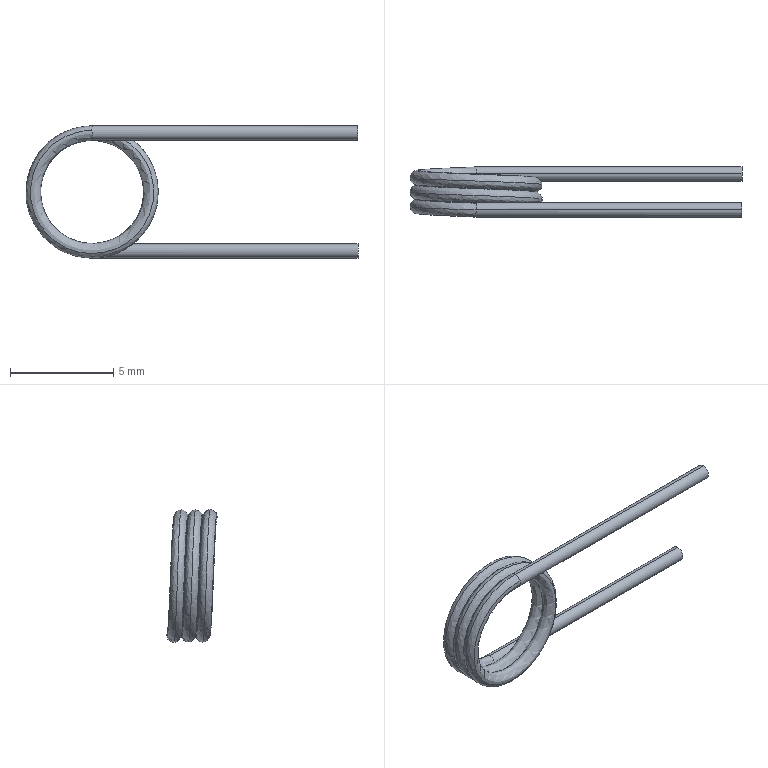Part | SolidWorks | features CompositeCurve 1, Helix 1, Sweep 1 | 1 solid | 9 faces | box 16.05 x 2.45 x 6.4 mm | volume 26.63 mm3 | cylinder 4 | spline 3 | plane 2 | commonest cylinder face diameters 0.7 x4
STEP:
#1=CARTESIAN_POINT('',(12.85,1.75,-3.2));
#2=VERTEX_POINT('',#1);
#3=CARTESIAN_POINT('',(12.85,1.75,-2.5));
#4=VERTEX_POINT('',#3);
#5=CARTESIAN_POINT('',(12.85,1.75,-2.85));
#6=DIRECTION('',(1.,0.,0.));
#7=DIRECTION('',(0.,0.00009155,-1.));
#8=AXIS2_PLACEMENT_3D('',#5,#6,#7);
#9=CIRCLE('',#8,0.35);
#10=EDGE_CURVE('',#2,#4,#9,.T.);
#11=ORIENTED_EDGE('',*,*,#10,.F.);
#12=CARTESIAN_POINT('',(-0.000000536,1.75,-3.2));
#13=VERTEX_POINT('',#12);
#14=CARTESIAN_POINT('',(12.85,1.75,-3.2));
#15=DIRECTION('',(-1.,0.,0.));
#16=VECTOR('',#15,1000.);
#17=LINE('',#14,#16);
#18=EDGE_CURVE('',#2,#13,#17,.T.);
#19=ORIENTED_EDGE('',*,*,#18,.T.);
#20=CARTESIAN_POINT('',(-0.006305,2.074,-2.979));
#21=VERTEX_POINT('',#20);
#22=CARTESIAN_POINT('',(0.,1.75,-2.85));
#23=DIRECTION('',(1.,0.,0.));
#24=DIRECTION('',(0.,0.00009155,-1.));
#25=AXIS2_PLACEMENT_3D('',#22,#23,#24);
#26=CIRCLE('',#25,0.35);
#27=EDGE_CURVE('',#13,#21,#26,.T.);
#28=ORIENTED_EDGE('',*,*,#27,.T.);
#29=CARTESIAN_POINT('',(0.,1.75,-2.5));
#30=VERTEX_POINT('',#29);
#31=CARTESIAN_POINT('',(0.,1.75,-2.85));
#32=DIRECTION('',(1.,0.,0.));
#33=DIRECTION('',(0.,0.00009155,-1.));
#34=AXIS2_PLACEMENT_3D('',#31,#32,#33);
#35=CIRCLE('',#34,0.35);
#36=EDGE_CURVE('',#21,#30,#35,.T.);
#37=ORIENTED_EDGE('',*,*,#36,.T.);
#38=CARTESIAN_POINT('',(12.85,1.75,-2.5));
#39=DIRECTION('',(-1.,0.,0.));
#40=VECTOR('',#39,1000.);
#41=LINE('',#38,#40);
#42=EDGE_CURVE('',#4,#30,#41,.T.);
#43=ORIENTED_EDGE('',*,*,#42,.F.);
#44=EDGE_LOOP('',(#11,#19,#28,#37,#43));
#45=FACE_OUTER_BOUND('',#44,.T.);
#46=CARTESIAN_POINT('',(12.85,1.75,-2.85));
#47=DIRECTION('',(-1.,0.,0.));
#48=DIRECTION('',(0.,0.,1.));
#49=AXIS2_PLACEMENT_3D('',#46,#47,#48);
#50=CYLINDRICAL_SURFACE('',#49,0.35);
#51=ADVANCED_FACE('',(#45),#50,.T.);
#52=CARTESIAN_POINT('',(0.006305,0.3239,2.979));
#53=VERTEX_POINT('',#52);
#54=CARTESIAN_POINT('',(0.,0.,3.2));
#55=VERTEX_POINT('',#54);
#56=CARTESIAN_POINT('',(0.006305,0.3239,2.979));
#57=CARTESIAN_POINT('',(0.01048,0.2681,3.104));
#58=CARTESIAN_POINT('',(0.005425,0.1388,3.2));
#59=CARTESIAN_POINT('',(0.,0.,3.2));
#60=B_SPLINE_CURVE_WITH_KNOTS('',3,(#56,#57,#58,#59),.UNSPECIFIED.,.F.,.F.,(4,4),(0.00002721,0.1895),.UNSPECIFIED.);
#61=EDGE_CURVE('',#53,#55,#60,.T.);
#62=ORIENTED_EDGE('',*,*,#61,.T.);
#63=CARTESIAN_POINT('',(12.85,0.,3.2));
#64=VERTEX_POINT('',#63);
#65=CARTESIAN_POINT('',(0.,0.,3.2));
#66=DIRECTION('',(1.,0.,0.));
#67=VECTOR('',#66,1000.);
#68=LINE('',#65,#67);
#69=EDGE_CURVE('',#55,#64,#68,.T.);
#70=ORIENTED_EDGE('',*,*,#69,.T.);
#71=CARTESIAN_POINT('',(12.85,0.,2.5));
#72=VERTEX_POINT('',#71);
#73=CARTESIAN_POINT('',(12.85,0.,2.85));
#74=DIRECTION('',(-1.,0.,0.));
#75=DIRECTION('',(0.,0.,1.));
#76=AXIS2_PLACEMENT_3D('',#73,#74,#75);
#77=CIRCLE('',#76,0.35);
#78=EDGE_CURVE('',#64,#72,#77,.T.);
#79=ORIENTED_EDGE('',*,*,#78,.T.);
#80=CARTESIAN_POINT('',(0.,0.,2.5));
#81=VERTEX_POINT('',#80);
#82=CARTESIAN_POINT('',(0.,0.,2.5));
#83=DIRECTION('',(1.,0.,0.));
#84=VECTOR('',#83,1000.);
#85=LINE('',#82,#84);
#86=EDGE_CURVE('',#81,#72,#85,.T.);
#87=ORIENTED_EDGE('',*,*,#86,.F.);
#88=CARTESIAN_POINT('',(0.,0.,2.85));
#89=DIRECTION('',(-1.,0.,0.));
#90=DIRECTION('',(0.,0.,1.));
#91=AXIS2_PLACEMENT_3D('',#88,#89,#90);
#92=CIRCLE('',#91,0.35);
#93=EDGE_CURVE('',#53,#81,#92,.T.);
#94=ORIENTED_EDGE('',*,*,#93,.F.);
#95=EDGE_LOOP('',(#62,#70,#79,#87,#94));
#96=FACE_OUTER_BOUND('',#95,.T.);
#97=CARTESIAN_POINT('',(0.,0.,2.85));
#98=DIRECTION('',(1.,0.,0.));
#99=DIRECTION('',(0.,0.,-1.));
#100=AXIS2_PLACEMENT_3D('',#97,#98,#99);
#101=CYLINDRICAL_SURFACE('',#100,0.35);
#102=ADVANCED_FACE('',(#96),#101,.T.);
#103=ORIENTED_EDGE('',*,*,#18,.F.);
#104=CARTESIAN_POINT('',(12.85,1.75,-2.85));
#105=DIRECTION('',(1.,0.,0.));
#106=DIRECTION('',(0.,0.00009155,-1.));
#107=AXIS2_PLACEMENT_3D('',#104,#105,#106);
#108=CIRCLE('',#107,0.35);
#109=EDGE_CURVE('',#4,#2,#108,.T.);
#110=ORIENTED_EDGE('',*,*,#109,.F.);
#111=ORIENTED_EDGE('',*,*,#42,.T.);
#112=CARTESIAN_POINT('',(0.006304,1.426,-2.979));
#113=VERTEX_POINT('',#112);
#114=CARTESIAN_POINT('',(0.,1.75,-2.85));
#115=DIRECTION('',(1.,0.,0.));
#116=DIRECTION('',(0.,0.00009155,-1.));
#117=AXIS2_PLACEMENT_3D('',#114,#115,#116);
#118=CIRCLE('',#117,0.35);
#119=EDGE_CURVE('',#30,#113,#118,.T.);
#120=ORIENTED_EDGE('',*,*,#119,.T.);
#121=CARTESIAN_POINT('',(0.,1.75,-2.85));
#122=DIRECTION('',(1.,0.,0.));
#123=DIRECTION('',(0.,0.00009155,-1.));
#124=AXIS2_PLACEMENT_3D('',#121,#122,#123);
#125=CIRCLE('',#124,0.35);
#126=EDGE_CURVE('',#113,#13,#125,.T.);
#127=ORIENTED_EDGE('',*,*,#126,.T.);
#128=EDGE_LOOP('',(#103,#110,#111,#120,#127));
#129=FACE_OUTER_BOUND('',#128,.T.);
#130=CARTESIAN_POINT('',(12.85,1.75,-2.85));
#131=DIRECTION('',(-1.,0.,0.));
#132=DIRECTION('',(0.,0.,1.));
#133=AXIS2_PLACEMENT_3D('',#130,#131,#132);
#134=CYLINDRICAL_SURFACE('',#133,0.35);
#135=ADVANCED_FACE('',(#129),#134,.T.);
#136=ORIENTED_EDGE('',*,*,#36,.F.);
#137=CARTESIAN_POINT('',(0.006305,0.3239,2.979));
#138=CARTESIAN_POINT('',(-0.7712,0.3519,2.981));
#139=CARTESIAN_POINT('',(-1.545,0.381,2.663));
#140=CARTESIAN_POINT('',(-2.649,0.4392,1.566));
#141=CARTESIAN_POINT('',(-2.975,0.4683,0.7939));
#142=CARTESIAN_POINT('',(-2.98,0.5195,-0.5733));
#143=CARTESIAN_POINT('',(-2.806,0.5413,-1.156));
#144=CARTESIAN_POINT('',(-2.162,0.585,-2.13));
#145=CARTESIAN_POINT('',(-1.69,0.6069,-2.521));
#146=CARTESIAN_POINT('',(-0.4324,0.658,-3.048));
#147=CARTESIAN_POINT('',(0.405,0.6871,-3.052));
#148=CARTESIAN_POINT('',(1.67,0.7383,-2.534));
#149=CARTESIAN_POINT('',(2.142,0.7601,-2.15));
#150=CARTESIAN_POINT('',(2.795,0.8037,-1.182));
#151=CARTESIAN_POINT('',(2.976,0.8257,-0.5972));
#152=CARTESIAN_POINT('',(2.981,0.8768,0.7668));
#153=CARTESIAN_POINT('',(2.665,0.9058,1.542));
#154=CARTESIAN_POINT('',(1.702,0.957,2.513));
#155=CARTESIAN_POINT('',(1.167,0.9788,2.801));
#156=CARTESIAN_POINT('',(0.02248,1.022,3.035));
#157=CARTESIAN_POINT('',(-0.587,1.044,2.978));
#158=CARTESIAN_POINT('',(-1.849,1.096,2.461));
#159=CARTESIAN_POINT('',(-2.445,1.125,1.872));
#160=CARTESIAN_POINT('',(-2.973,1.176,0.6109));
#161=CARTESIAN_POINT('',(-3.035,1.198,0.005944));
#162=CARTESIAN_POINT('',(-2.812,1.241,-1.14));
#163=CARTESIAN_POINT('',(-2.526,1.263,-1.682));
#164=CARTESIAN_POINT('',(-1.566,1.314,-2.65));
#165=CARTESIAN_POINT('',(-0.7938,1.343,-2.975));
#166=CARTESIAN_POINT('',(0.5733,1.395,-2.98));
#167=CARTESIAN_POINT('',(1.156,1.416,-2.806));
#168=CARTESIAN_POINT('',(2.13,1.46,-2.162));
#169=CARTESIAN_POINT('',(2.521,1.482,-1.69));
#170=CARTESIAN_POINT('',(3.048,1.533,-0.4324));
#171=CARTESIAN_POINT('',(3.052,1.562,0.405));
#172=CARTESIAN_POINT('',(2.534,1.613,1.67));
#173=CARTESIAN_POINT('',(2.15,1.635,2.142));
#174=CARTESIAN_POINT('',(1.182,1.679,2.795));
#175=CARTESIAN_POINT('',(0.5972,1.701,2.976));
#176=CARTESIAN_POINT('',(-0.7668,1.752,2.981));
#177=CARTESIAN_POINT('',(-1.542,1.781,2.665));
#178=CARTESIAN_POINT('',(-2.513,1.832,1.702));
#179=CARTESIAN_POINT('',(-2.801,1.854,1.167));
#180=CARTESIAN_POINT('',(-3.034,1.897,0.0225));
#181=CARTESIAN_POINT('',(-2.978,1.919,-0.587));
#182=CARTESIAN_POINT('',(-2.46,1.971,-1.85));
#183=CARTESIAN_POINT('',(-1.872,2.,-2.445));
#184=CARTESIAN_POINT('',(-0.7917,2.043,-2.897));
#185=CARTESIAN_POINT('',(-0.4042,2.058,-2.976));
#186=CARTESIAN_POINT('',(-0.006305,2.074,-2.979));
#187=B_SPLINE_CURVE_WITH_KNOTS('',3,(#137,#138,#139,#140,#141,#142,#143,#144,#145,#146,#147,#148,#149,#150,#151,#152,#153,#154,#155,#156,#157,#158,#159,#160,#161,#162,#163,#164,#165,#166,#167,#168,#169,#170,#171,#172,#173,#174,#175,#176,#177,#178,#179,#180,#181,#182,#183,#184,#185,#186),.UNSPECIFIED.,.F.,.F.,(4,2,2,2,2,2,2,2,2,2,2,2,2,2,2,2,2,2,2,2,2,2,2,2,4),(0.,0.04998,0.09999,0.1375,0.175,0.225,0.2625,0.3,0.35,0.3875,0.425,0.475,0.5125,0.55,0.6,0.6375,0.675,0.725,0.7625,0.8,0.85,0.8875,0.925,0.975,1.),.UNSPECIFIED.);
#188=EDGE_CURVE('',#53,#21,#187,.T.);
#189=ORIENTED_EDGE('',*,*,#188,.F.);
#190=ORIENTED_EDGE('',*,*,#93,.T.);
#191=CARTESIAN_POINT('',(-0.006304,-0.3239,2.979));
#192=VERTEX_POINT('',#191);
#193=CARTESIAN_POINT('',(0.,0.,2.85));
#194=DIRECTION('',(-1.,0.,0.));
#195=DIRECTION('',(0.,0.,1.));
#196=AXIS2_PLACEMENT_3D('',#193,#194,#195);
#197=CIRCLE('',#196,0.35);
#198=EDGE_CURVE('',#81,#192,#197,.T.);
#199=ORIENTED_EDGE('',*,*,#198,.T.);
#200=CARTESIAN_POINT('',(0.006304,1.426,-2.979));
#201=CARTESIAN_POINT('',(-0.379,1.413,-2.98));
#202=CARTESIAN_POINT('',(-0.7673,1.398,-2.904));
#203=CARTESIAN_POINT('',(-1.851,1.354,-2.461));
#204=CARTESIAN_POINT('',(-2.445,1.325,-1.871));
#205=CARTESIAN_POINT('',(-2.973,1.274,-0.6122));
#206=CARTESIAN_POINT('',(-3.035,1.252,-0.003211));
#207=CARTESIAN_POINT('',(-2.811,1.209,1.143));
#208=CARTESIAN_POINT('',(-2.527,1.187,1.681));
#209=CARTESIAN_POINT('',(-1.565,1.136,2.652));
#210=CARTESIAN_POINT('',(-0.792,1.107,2.975));
#211=CARTESIAN_POINT('',(0.572,1.056,2.981));
#212=CARTESIAN_POINT('',(1.158,1.034,2.805));
#213=CARTESIAN_POINT('',(2.132,0.99,2.16));
#214=CARTESIAN_POINT('',(2.52,0.9682,1.692));
#215=CARTESIAN_POINT('',(3.049,0.917,0.4308));
#216=CARTESIAN_POINT('',(3.052,0.8879,-0.4067));
#217=CARTESIAN_POINT('',(2.535,0.8368,-1.669));
#218=CARTESIAN_POINT('',(2.148,0.8149,-2.144));
#219=CARTESIAN_POINT('',(1.18,0.7712,-2.796));
#220=CARTESIAN_POINT('',(0.5985,0.7494,-2.976));
#221=CARTESIAN_POINT('',(-0.7686,0.6982,-2.981));
#222=CARTESIAN_POINT('',(-1.544,0.6692,-2.664));
#223=CARTESIAN_POINT('',(-2.512,0.6181,-1.703));
#224=CARTESIAN_POINT('',(-2.802,0.5961,-1.164));
#225=CARTESIAN_POINT('',(-3.035,0.5525,-0.01977));
#226=CARTESIAN_POINT('',(-2.978,0.5307,0.5858));
#227=CARTESIAN_POINT('',(-2.46,0.4795,1.851));
#228=CARTESIAN_POINT('',(-1.87,0.4504,2.445));
#229=CARTESIAN_POINT('',(-0.6122,0.3993,2.973));
#230=CARTESIAN_POINT('',(-0.003226,0.3774,3.035));
#231=CARTESIAN_POINT('',(1.143,0.3337,2.811));
#232=CARTESIAN_POINT('',(1.681,0.3119,2.527));
#233=CARTESIAN_POINT('',(2.652,0.2607,1.565));
#234=CARTESIAN_POINT('',(2.975,0.2317,0.792));
#235=CARTESIAN_POINT('',(2.981,0.1806,-0.572));
#236=CARTESIAN_POINT('',(2.805,0.1586,-1.158));
#237=CARTESIAN_POINT('',(2.16,0.115,-2.132));
#238=CARTESIAN_POINT('',(1.692,0.09317,-2.52));
#239=CARTESIAN_POINT('',(0.4308,0.04196,-3.049));
#240=CARTESIAN_POINT('',(-0.4067,0.01292,-3.052));
#241=CARTESIAN_POINT('',(-1.669,-0.03818,-2.535));
#242=CARTESIAN_POINT('',(-2.144,-0.06013,-2.148));
#243=CARTESIAN_POINT('',(-2.796,-0.1038,-1.18));
#244=CARTESIAN_POINT('',(-2.976,-0.1256,-0.5985));
#245=CARTESIAN_POINT('',(-2.981,-0.1768,0.7687));
#246=CARTESIAN_POINT('',(-2.663,-0.2059,1.544));
#247=CARTESIAN_POINT('',(-1.567,-0.2642,2.65));
#248=CARTESIAN_POINT('',(-0.7966,-0.2932,2.975));
#249=CARTESIAN_POINT('',(-0.006304,-0.3239,2.979));
#250=B_SPLINE_CURVE_WITH_KNOTS('',3,(#200,#201,#202,#203,#204,#205,#206,#207,#208,#209,#210,#211,#212,#213,#214,#215,#216,#217,#218,#219,#220,#221,#222,#223,#224,#225,#226,#227,#228,#229,#230,#231,#232,#233,#234,#235,#236,#237,#238,#239,#240,#241,#242,#243,#244,#245,#246,#247,#248,#249),.UNSPECIFIED.,.F.,.F.,(4,2,2,2,2,2,2,2,2,2,2,2,2,2,2,2,2,2,2,2,2,2,2,2,4),(0.,0.02496,0.07501,0.1125,0.15,0.2,0.2375,0.275,0.325,0.3625,0.4,0.45,0.4875,0.525,0.575,0.6125,0.65,0.7,0.7375,0.775,0.825,0.8625,0.9,0.95,1.),.UNSPECIFIED.);
#251=EDGE_CURVE('',#113,#192,#250,.T.);
#252=ORIENTED_EDGE('',*,*,#251,.F.);
#253=ORIENTED_EDGE('',*,*,#119,.F.);
#254=EDGE_LOOP('',(#136,#189,#190,#199,#252,#253));
#255=FACE_OUTER_BOUND('',#254,.T.);
#256=CARTESIAN_POINT('',(-0.01261,2.073,-2.978));
#257=CARTESIAN_POINT('',(-0.9931,2.036,-2.974));
#258=CARTESIAN_POINT('',(-1.942,2.,-2.452));
#259=CARTESIAN_POINT('',(-3.022,1.927,-0.8338));
#260=CARTESIAN_POINT('',(-3.123,1.89,0.2539));
#261=CARTESIAN_POINT('',(-2.369,1.817,2.048));
#262=CARTESIAN_POINT('',(-1.523,1.781,2.732));
#263=CARTESIAN_POINT('',(0.3864,1.708,3.111));
#264=CARTESIAN_POINT('',(1.43,1.671,2.788));
#265=CARTESIAN_POINT('',(2.798,1.599,1.405));
#266=CARTESIAN_POINT('',(3.107,1.562,0.3615));
#267=CARTESIAN_POINT('',(2.726,1.489,-1.547));
#268=CARTESIAN_POINT('',(2.029,1.453,-2.388));
#269=CARTESIAN_POINT('',(0.2273,1.38,-3.123));
#270=CARTESIAN_POINT('',(-0.8551,1.343,-3.009));
#271=CARTESIAN_POINT('',(-2.473,1.271,-1.927));
#272=CARTESIAN_POINT('',(-2.982,1.234,-0.9604));
#273=CARTESIAN_POINT('',(-2.972,1.161,0.9852));
#274=CARTESIAN_POINT('',(-2.453,1.125,1.942));
#275=CARTESIAN_POINT('',(-0.8335,1.052,3.022));
#276=CARTESIAN_POINT('',(0.2539,1.015,3.123));
#277=CARTESIAN_POINT('',(2.048,0.9425,2.369));
#278=CARTESIAN_POINT('',(2.732,0.9059,1.523));
#279=CARTESIAN_POINT('',(3.111,0.8331,-0.3864));
#280=CARTESIAN_POINT('',(2.788,0.7965,-1.43));
#281=CARTESIAN_POINT('',(1.405,0.7237,-2.798));
#282=CARTESIAN_POINT('',(0.3615,0.6872,-3.107));
#283=CARTESIAN_POINT('',(-1.547,0.6143,-2.726));
#284=CARTESIAN_POINT('',(-2.388,0.5777,-2.029));
#285=CARTESIAN_POINT('',(-3.123,0.505,-0.2273));
#286=CARTESIAN_POINT('',(-3.009,0.4684,0.8554));
#287=CARTESIAN_POINT('',(-1.927,0.3956,2.473));
#288=CARTESIAN_POINT('',(-0.9676,0.3593,2.982));
#289=CARTESIAN_POINT('',(0.01261,0.3226,2.978));
#290=CARTESIAN_POINT('',(-0.0161,2.162,-2.771));
#291=CARTESIAN_POINT('',(-0.9269,2.125,-2.766));
#292=CARTESIAN_POINT('',(-1.811,2.089,-2.279));
#293=CARTESIAN_POINT('',(-2.813,2.016,-0.7712));
#294=CARTESIAN_POINT('',(-2.906,1.979,0.2409));
#295=CARTESIAN_POINT('',(-2.201,1.907,1.909));
#296=CARTESIAN_POINT('',(-1.413,1.87,2.545));
#297=CARTESIAN_POINT('',(0.3644,1.797,2.894));
#298=CARTESIAN_POINT('',(1.334,1.761,2.592));
#299=CARTESIAN_POINT('',(2.606,1.688,1.303));
#300=CARTESIAN_POINT('',(2.892,1.651,0.3318));
#301=CARTESIAN_POINT('',(2.535,1.579,-1.444));
#302=CARTESIAN_POINT('',(1.884,1.542,-2.225));
#303=CARTESIAN_POINT('',(0.2064,1.469,-2.907));
#304=CARTESIAN_POINT('',(-0.8001,1.433,-2.799));
#305=CARTESIAN_POINT('',(-2.304,1.36,-1.789));
#306=CARTESIAN_POINT('',(-2.777,1.323,-0.8894));
#307=CARTESIAN_POINT('',(-2.764,1.25,0.9216));
#308=CARTESIAN_POINT('',(-2.279,1.214,1.81));
#309=CARTESIAN_POINT('',(-0.771,1.141,2.814));
#310=CARTESIAN_POINT('',(0.2409,1.104,2.906));
#311=CARTESIAN_POINT('',(1.909,1.032,2.201));
#312=CARTESIAN_POINT('',(2.545,0.9951,1.413));
#313=CARTESIAN_POINT('',(2.894,0.9223,-0.3644));
#314=CARTESIAN_POINT('',(2.592,0.8857,-1.334));
#315=CARTESIAN_POINT('',(1.303,0.8129,-2.606));
#316=CARTESIAN_POINT('',(0.3318,0.7764,-2.892));
#317=CARTESIAN_POINT('',(-1.444,0.7035,-2.535));
#318=CARTESIAN_POINT('',(-2.225,0.667,-1.884));
#319=CARTESIAN_POINT('',(-2.907,0.5942,-0.2064));
#320=CARTESIAN_POINT('',(-2.798,0.5576,0.8003));
#321=CARTESIAN_POINT('',(-1.789,0.4848,2.304));
#322=CARTESIAN_POINT('',(-0.8958,0.4485,2.776));
#323=CARTESIAN_POINT('',(0.0161,0.4118,2.771));
#324=CARTESIAN_POINT('',(-0.008888,1.977,-2.5));
#325=CARTESIAN_POINT('',(-0.8283,1.941,-2.497));
#326=CARTESIAN_POINT('',(-1.629,1.904,-2.059));
#327=CARTESIAN_POINT('',(-2.536,1.832,-0.7012));
#328=CARTESIAN_POINT('',(-2.622,1.795,0.2114));
#329=CARTESIAN_POINT('',(-1.989,1.722,1.718));
#330=CARTESIAN_POINT('',(-1.28,1.686,2.292));
#331=CARTESIAN_POINT('',(0.3232,1.613,2.612));
#332=CARTESIAN_POINT('',(1.199,1.576,2.341));
#333=CARTESIAN_POINT('',(2.349,1.503,1.18));
#334=CARTESIAN_POINT('',(2.608,1.467,0.3051));
#335=CARTESIAN_POINT('',(2.29,1.394,-1.298));
#336=CARTESIAN_POINT('',(1.704,1.358,-2.003));
#337=CARTESIAN_POINT('',(0.1914,1.285,-2.622));
#338=CARTESIAN_POINT('',(-0.716,1.248,-2.526));
#339=CARTESIAN_POINT('',(-2.075,1.175,-1.618));
#340=CARTESIAN_POINT('',(-2.503,1.139,-0.808));
#341=CARTESIAN_POINT('',(-2.495,1.066,0.8264));
#342=CARTESIAN_POINT('',(-2.06,1.029,1.628));
#343=CARTESIAN_POINT('',(-0.701,0.9565,2.537));
#344=CARTESIAN_POINT('',(0.2114,0.92,2.622));
#345=CARTESIAN_POINT('',(1.718,0.8471,1.989));
#346=CARTESIAN_POINT('',(2.292,0.8107,1.28));
#347=CARTESIAN_POINT('',(2.612,0.7378,-0.3232));
#348=CARTESIAN_POINT('',(2.341,0.7013,-1.199));
#349=CARTESIAN_POINT('',(1.18,0.6284,-2.349));
#350=CARTESIAN_POINT('',(0.3051,0.5919,-2.608));
#351=CARTESIAN_POINT('',(-1.298,0.519,-2.29));
#352=CARTESIAN_POINT('',(-2.003,0.4825,-1.704));
#353=CARTESIAN_POINT('',(-2.622,0.4096,-0.1914));
#354=CARTESIAN_POINT('',(-2.525,0.3732,0.7162));
#355=CARTESIAN_POINT('',(-1.619,0.3003,2.075));
#356=CARTESIAN_POINT('',(-0.8134,0.2639,2.503));
#357=CARTESIAN_POINT('',(0.008889,0.2274,2.5));
#358=CARTESIAN_POINT('',(0.008895,1.522,-2.5));
#359=CARTESIAN_POINT('',(-0.8105,1.486,-2.503));
#360=CARTESIAN_POINT('',(-1.614,1.45,-2.071));
#361=CARTESIAN_POINT('',(-2.532,1.377,-0.7193));
#362=CARTESIAN_POINT('',(-2.623,1.34,0.1927));
#363=CARTESIAN_POINT('',(-2.001,1.267,1.704));
#364=CARTESIAN_POINT('',(-1.296,1.231,2.283));
#365=CARTESIAN_POINT('',(0.3046,1.158,2.614));
#366=CARTESIAN_POINT('',(1.182,1.121,2.35));
#367=CARTESIAN_POINT('',(2.341,1.048,1.197));
#368=CARTESIAN_POINT('',(2.606,1.012,0.3236));
#369=CARTESIAN_POINT('',(2.299,0.9391,-1.282));
#370=CARTESIAN_POINT('',(1.719,0.9026,-1.991));
#371=CARTESIAN_POINT('',(0.2101,0.8297,-2.62));
#372=CARTESIAN_POINT('',(-0.6981,0.7933,-2.531));
#373=CARTESIAN_POINT('',(-2.064,0.7204,-1.633));
#374=CARTESIAN_POINT('',(-2.497,0.6839,-0.8259));
#375=CARTESIAN_POINT('',(-2.501,0.611,0.8087));
#376=CARTESIAN_POINT('',(-2.071,0.5745,1.614));
#377=CARTESIAN_POINT('',(-0.7191,0.5016,2.532));
#378=CARTESIAN_POINT('',(0.1927,0.4651,2.623));
#379=CARTESIAN_POINT('',(1.704,0.3922,2.001));
#380=CARTESIAN_POINT('',(2.283,0.3558,1.296));
#381=CARTESIAN_POINT('',(2.614,0.2829,-0.3046));
#382=CARTESIAN_POINT('',(2.35,0.2464,-1.182));
#383=CARTESIAN_POINT('',(1.197,0.1735,-2.341));
#384=CARTESIAN_POINT('',(0.3236,0.137,-2.606));
#385=CARTESIAN_POINT('',(-1.282,0.0641,-2.299));
#386=CARTESIAN_POINT('',(-1.991,0.02763,-1.719));
#387=CARTESIAN_POINT('',(-2.62,-0.04528,-0.2101));
#388=CARTESIAN_POINT('',(-2.531,-0.08173,0.6983));
#389=CARTESIAN_POINT('',(-1.633,-0.1546,2.064));
#390=CARTESIAN_POINT('',(-0.8313,-0.191,2.497));
#391=CARTESIAN_POINT('',(-0.008894,-0.2275,2.5));
#392=CARTESIAN_POINT('',(0.0161,1.338,-2.771));
#393=CARTESIAN_POINT('',(-0.8947,1.302,-2.777));
#394=CARTESIAN_POINT('',(-1.785,1.265,-2.3));
#395=CARTESIAN_POINT('',(-2.804,1.192,-0.804));
#396=CARTESIAN_POINT('',(-2.908,1.156,0.2071));
#397=CARTESIAN_POINT('',(-2.223,1.083,1.884));
#398=CARTESIAN_POINT('',(-1.443,1.046,2.528));
#399=CARTESIAN_POINT('',(0.3307,0.9736,2.899));
#400=CARTESIAN_POINT('',(1.304,0.937,2.608));
#401=CARTESIAN_POINT('',(2.591,0.8642,1.333));
#402=CARTESIAN_POINT('',(2.888,0.8277,0.3653));
#403=CARTESIAN_POINT('',(2.552,0.7548,-1.415));
#404=CARTESIAN_POINT('',(1.91,0.7183,-2.203));
#405=CARTESIAN_POINT('',(0.2402,0.6455,-2.904));
#406=CARTESIAN_POINT('',(-0.7677,0.6089,-2.808));
#407=CARTESIAN_POINT('',(-2.284,0.5361,-1.816));
#408=CARTESIAN_POINT('',(-2.766,0.4995,-0.9217));
#409=CARTESIAN_POINT('',(-2.775,0.4267,0.8895));
#410=CARTESIAN_POINT('',(-2.3,0.3902,1.784));
#411=CARTESIAN_POINT('',(-0.8038,0.3173,2.805));
#412=CARTESIAN_POINT('',(0.2071,0.2808,2.908));
#413=CARTESIAN_POINT('',(1.884,0.208,2.223));
#414=CARTESIAN_POINT('',(2.528,0.1714,1.443));
#415=CARTESIAN_POINT('',(2.899,0.09857,-0.3307));
#416=CARTESIAN_POINT('',(2.608,0.06204,-1.304));
#417=CARTESIAN_POINT('',(1.333,-0.01079,-2.591));
#418=CARTESIAN_POINT('',(0.3653,-0.0473,-2.888));
#419=CARTESIAN_POINT('',(-1.415,-0.1202,-2.552));
#420=CARTESIAN_POINT('',(-2.203,-0.1567,-1.91));
#421=CARTESIAN_POINT('',(-2.904,-0.2295,-0.2402));
#422=CARTESIAN_POINT('',(-2.807,-0.2661,0.7679));
#423=CARTESIAN_POINT('',(-1.816,-0.3389,2.283));
#424=CARTESIAN_POINT('',(-0.9282,-0.3752,2.766));
#425=CARTESIAN_POINT('',(-0.0161,-0.4119,2.771));
#426=CARTESIAN_POINT('',(0.01261,1.427,-2.978));
#427=CARTESIAN_POINT('',(-0.9679,1.391,-2.982));
#428=CARTESIAN_POINT('',(-1.922,1.354,-2.469));
#429=CARTESIAN_POINT('',(-3.015,1.282,-0.8595));
#430=CARTESIAN_POINT('',(-3.125,1.245,0.2275));
#431=CARTESIAN_POINT('',(-2.386,1.172,2.028));
#432=CARTESIAN_POINT('',(-1.546,1.136,2.72));
#433=CARTESIAN_POINT('',(0.36,1.063,3.114));
#434=CARTESIAN_POINT('',(1.406,1.026,2.8));
#435=CARTESIAN_POINT('',(2.787,0.9536,1.429));
#436=CARTESIAN_POINT('',(3.104,0.917,0.3878));
#437=CARTESIAN_POINT('',(2.739,0.8442,-1.524));
#438=CARTESIAN_POINT('',(2.049,0.8076,-2.37));
#439=CARTESIAN_POINT('',(0.2537,0.7349,-3.121));
#440=CARTESIAN_POINT('',(-0.8297,0.6983,-3.016));
#441=CARTESIAN_POINT('',(-2.457,0.6254,-1.948));
#442=CARTESIAN_POINT('',(-2.974,0.5889,-0.9857));
#443=CARTESIAN_POINT('',(-2.981,0.5161,0.96));
#444=CARTESIAN_POINT('',(-2.469,0.4795,1.921));
#445=CARTESIAN_POINT('',(-0.8592,0.4067,3.015));
#446=CARTESIAN_POINT('',(0.2275,0.3701,3.125));
#447=CARTESIAN_POINT('',(2.028,0.2974,2.386));
#448=CARTESIAN_POINT('',(2.72,0.2608,1.546));
#449=CARTESIAN_POINT('',(3.114,0.1879,-0.36));
#450=CARTESIAN_POINT('',(2.8,0.1514,-1.406));
#451=CARTESIAN_POINT('',(1.429,0.07861,-2.787));
#452=CARTESIAN_POINT('',(0.3878,0.04204,-3.104));
#453=CARTESIAN_POINT('',(-1.524,-0.03081,-2.739));
#454=CARTESIAN_POINT('',(-2.371,-0.06738,-2.049));
#455=CARTESIAN_POINT('',(-3.121,-0.1401,-0.2537));
#456=CARTESIAN_POINT('',(-3.016,-0.1767,0.83));
#457=CARTESIAN_POINT('',(-1.948,-0.2496,2.456));
#458=CARTESIAN_POINT('',(-0.993,-0.2858,2.974));
#459=CARTESIAN_POINT('',(-0.01261,-0.3225,2.978));
#460=B_SPLINE_SURFACE_WITH_KNOTS('',3,3,((#256,#257,#258,#259,#260,#261,#262,#263,#264,#265,#266,#267,#268,#269,#270,#271,#272,#273,#274,#275,#276,#277,#278,#279,#280,#281,#282,#283,#284,#285,#286,#287,#288,#289),(#290,#291,#292,#293,#294,#295,#296,#297,#298,#299,#300,#301,#302,#303,#304,#305,#306,#307,#308,#309,#310,#311,#312,#313,#314,#315,#316,#317,#318,#319,#320,#321,#322,#323),(#324,#325,#326,#327,#328,#329,#330,#331,#332,#333,#334,#335,#336,#337,#338,#339,#340,#341,#342,#343,#344,#345,#346,#347,#348,#349,#350,#351,#352,#353,#354,#355,#356,#357),(#358,#359,#360,#361,#362,#363,#364,#365,#366,#367,#368,#369,#370,#371,#372,#373,#374,#375,#376,#377,#378,#379,#380,#381,#382,#383,#384,#385,#386,#387,#388,#389,#390,#391),(#392,#393,#394,#395,#396,#397,#398,#399,#400,#401,#402,#403,#404,#405,#406,#407,#408,#409,#410,#411,#412,#413,#414,#415,#416,#417,#418,#419,#420,#421,#422,#423,#424,#425),(#426,#427,#428,#429,#430,#431,#432,#433,#434,#435,#436,#437,#438,#439,#440,#441,#442,#443,#444,#445,#446,#447,#448,#449,#450,#451,#452,#453,#454,#455,#456,#457,#458,#459)),.UNSPECIFIED.,.F.,.F.,.F.,(4,2,4),(4,2,2,2,2,2,2,2,2,2,2,2,2,2,2,2,4),(0.1895,0.5,0.8106),(0.,0.0625,0.125,0.1875,0.25,0.3125,0.375,0.4375,0.5,0.5625,0.625,0.6875,0.75,0.8125,0.875,0.9375,1.),.UNSPECIFIED.);
#461=ADVANCED_FACE('',(#255),#460,.F.);
#462=ORIENTED_EDGE('',*,*,#126,.F.);
#463=ORIENTED_EDGE('',*,*,#251,.T.);
#464=CARTESIAN_POINT('',(0.,0.,3.2));
#465=CARTESIAN_POINT('',(-0.005423,-0.1387,3.2));
#466=CARTESIAN_POINT('',(-0.01048,-0.268,3.104));
#467=CARTESIAN_POINT('',(-0.006304,-0.3239,2.979));
#468=B_SPLINE_CURVE_WITH_KNOTS('',3,(#464,#465,#466,#467),.UNSPECIFIED.,.F.,.F.,(4,4),(0.8106,1.),.UNSPECIFIED.);
#469=EDGE_CURVE('',#55,#192,#468,.T.);
#470=ORIENTED_EDGE('',*,*,#469,.F.);
#471=CARTESIAN_POINT('',(-0.000000536,1.75,-3.2));
#472=CARTESIAN_POINT('',(-0.4215,1.735,-3.2));
#473=CARTESIAN_POINT('',(-0.8371,1.721,-3.117));
#474=CARTESIAN_POINT('',(-2.001,1.677,-2.635));
#475=CARTESIAN_POINT('',(-2.635,1.648,-2.));
#476=CARTESIAN_POINT('',(-3.197,1.597,-0.6438));
#477=CARTESIAN_POINT('',(-3.261,1.575,0.01064));
#478=CARTESIAN_POINT('',(-3.015,1.531,1.241));
#479=CARTESIAN_POINT('',(-2.708,1.51,1.817));
#480=CARTESIAN_POINT('',(-1.669,1.458,2.857));
#481=CARTESIAN_POINT('',(-0.8382,1.429,3.2));
#482=CARTESIAN_POINT('',(0.6287,1.378,3.2));
#483=CARTESIAN_POINT('',(1.258,1.356,3.008));
#484=CARTESIAN_POINT('',(2.3,1.313,2.311));
#485=CARTESIAN_POINT('',(2.715,1.291,1.807));
#486=CARTESIAN_POINT('',(3.278,1.239,0.4484));
#487=CARTESIAN_POINT('',(3.277,1.211,-0.4502));
#488=CARTESIAN_POINT('',(2.716,1.159,-1.805));
#489=CARTESIAN_POINT('',(2.298,1.137,-2.313));
#490=CARTESIAN_POINT('',(1.255,1.094,-3.01));
#491=CARTESIAN_POINT('',(0.6301,1.072,-3.2));
#492=CARTESIAN_POINT('',(-0.8402,1.021,-3.2));
#493=CARTESIAN_POINT('',(-1.67,0.9918,-2.855));
#494=CARTESIAN_POINT('',(-2.707,0.9406,-1.818));
#495=CARTESIAN_POINT('',(-3.017,0.9186,-1.238));
#496=CARTESIAN_POINT('',(-3.261,0.875,-0.007701));
#497=CARTESIAN_POINT('',(-3.198,0.8533,0.6424));
#498=CARTESIAN_POINT('',(-2.635,0.8019,2.001));
#499=CARTESIAN_POINT('',(-1.999,0.773,2.636));
#500=CARTESIAN_POINT('',(-0.6438,0.7218,3.197));
#501=CARTESIAN_POINT('',(0.01062,0.6999,3.261));
#502=CARTESIAN_POINT('',(1.241,0.6563,3.015));
#503=CARTESIAN_POINT('',(1.817,0.6345,2.708));
#504=CARTESIAN_POINT('',(2.857,0.5832,1.669));
#505=CARTESIAN_POINT('',(3.2,0.5543,0.8382));
#506=CARTESIAN_POINT('',(3.2,0.5031,-0.6287));
#507=CARTESIAN_POINT('',(3.008,0.4811,-1.258));
#508=CARTESIAN_POINT('',(2.311,0.4375,-2.3));
#509=CARTESIAN_POINT('',(1.807,0.4158,-2.715));
#510=CARTESIAN_POINT('',(0.4484,0.3644,-3.278));
#511=CARTESIAN_POINT('',(-0.4502,0.3355,-3.277));
#512=CARTESIAN_POINT('',(-1.805,0.2843,-2.716));
#513=CARTESIAN_POINT('',(-2.313,0.2624,-2.298));
#514=CARTESIAN_POINT('',(-3.01,0.2188,-1.255));
#515=CARTESIAN_POINT('',(-3.2,0.197,-0.6301));
#516=CARTESIAN_POINT('',(-3.2,0.1457,0.8403));
#517=CARTESIAN_POINT('',(-2.854,0.1167,1.671));
#518=CARTESIAN_POINT('',(-1.671,0.05831,2.854));
#519=CARTESIAN_POINT('',(-0.8425,0.02943,3.2));
#520=CARTESIAN_POINT('',(0.,0.,3.2));
#521=B_SPLINE_CURVE_WITH_KNOTS('',3,(#471,#472,#473,#474,#475,#476,#477,#478,#479,#480,#481,#482,#483,#484,#485,#486,#487,#488,#489,#490,#491,#492,#493,#494,#495,#496,#497,#498,#499,#500,#501,#502,#503,#504,#505,#506,#507,#508,#509,#510,#511,#512,#513,#514,#515,#516,#517,#518,#519,#520),.UNSPECIFIED.,.F.,.F.,(4,2,2,2,2,2,2,2,2,2,2,2,2,2,2,2,2,2,2,2,2,2,2,2,4),(0.,0.02496,0.07501,0.1125,0.15,0.2,0.2375,0.275,0.325,0.3625,0.4,0.45,0.4875,0.525,0.575,0.6125,0.65,0.7,0.7375,0.775,0.825,0.8625,0.9,0.95,1.),.UNSPECIFIED.);
#522=EDGE_CURVE('',#13,#55,#521,.T.);
#523=ORIENTED_EDGE('',*,*,#522,.F.);
#524=EDGE_LOOP('',(#462,#463,#470,#523));
#525=FACE_OUTER_BOUND('',#524,.T.);
#526=CARTESIAN_POINT('',(0.01261,1.427,-2.978));
#527=CARTESIAN_POINT('',(-0.379,1.413,-2.98));
#528=CARTESIAN_POINT('',(-0.7673,1.398,-2.904));
#529=CARTESIAN_POINT('',(-1.851,1.354,-2.461));
#530=CARTESIAN_POINT('',(-2.445,1.325,-1.871));
#531=CARTESIAN_POINT('',(-2.973,1.274,-0.6122));
#532=CARTESIAN_POINT('',(-3.035,1.252,-0.003211));
#533=CARTESIAN_POINT('',(-2.811,1.209,1.143));
#534=CARTESIAN_POINT('',(-2.527,1.187,1.681));
#535=CARTESIAN_POINT('',(-1.565,1.136,2.652));
#536=CARTESIAN_POINT('',(-0.792,1.107,2.975));
#537=CARTESIAN_POINT('',(0.572,1.056,2.981));
#538=CARTESIAN_POINT('',(1.158,1.034,2.805));
#539=CARTESIAN_POINT('',(2.132,0.99,2.16));
#540=CARTESIAN_POINT('',(2.52,0.9682,1.692));
#541=CARTESIAN_POINT('',(3.049,0.917,0.4308));
#542=CARTESIAN_POINT('',(3.052,0.8879,-0.4067));
#543=CARTESIAN_POINT('',(2.535,0.8368,-1.669));
#544=CARTESIAN_POINT('',(2.148,0.8149,-2.144));
#545=CARTESIAN_POINT('',(1.18,0.7712,-2.796));
#546=CARTESIAN_POINT('',(0.5985,0.7494,-2.976));
#547=CARTESIAN_POINT('',(-0.7686,0.6982,-2.981));
#548=CARTESIAN_POINT('',(-1.544,0.6692,-2.664));
#549=CARTESIAN_POINT('',(-2.512,0.6181,-1.703));
#550=CARTESIAN_POINT('',(-2.802,0.5961,-1.164));
#551=CARTESIAN_POINT('',(-3.035,0.5525,-0.01977));
#552=CARTESIAN_POINT('',(-2.978,0.5307,0.5858));
#553=CARTESIAN_POINT('',(-2.46,0.4795,1.851));
#554=CARTESIAN_POINT('',(-1.87,0.4504,2.445));
#555=CARTESIAN_POINT('',(-0.6122,0.3993,2.973));
#556=CARTESIAN_POINT('',(-0.003226,0.3774,3.035));
#557=CARTESIAN_POINT('',(1.143,0.3337,2.811));
#558=CARTESIAN_POINT('',(1.681,0.3119,2.527));
#559=CARTESIAN_POINT('',(2.652,0.2607,1.565));
#560=CARTESIAN_POINT('',(2.975,0.2317,0.792));
#561=CARTESIAN_POINT('',(2.981,0.1806,-0.572));
#562=CARTESIAN_POINT('',(2.805,0.1586,-1.158));
#563=CARTESIAN_POINT('',(2.16,0.115,-2.132));
#564=CARTESIAN_POINT('',(1.692,0.09317,-2.52));
#565=CARTESIAN_POINT('',(0.4308,0.04196,-3.049));
#566=CARTESIAN_POINT('',(-0.4067,0.01292,-3.052));
#567=CARTESIAN_POINT('',(-1.669,-0.03818,-2.535));
#568=CARTESIAN_POINT('',(-2.144,-0.06013,-2.148));
#569=CARTESIAN_POINT('',(-2.796,-0.1038,-1.18));
#570=CARTESIAN_POINT('',(-2.976,-0.1256,-0.5985));
#571=CARTESIAN_POINT('',(-2.981,-0.1768,0.7687));
#572=CARTESIAN_POINT('',(-2.663,-0.2059,1.544));
#573=CARTESIAN_POINT('',(-1.567,-0.2642,2.65));
#574=CARTESIAN_POINT('',(-0.7966,-0.2932,2.975));
#575=CARTESIAN_POINT('',(-0.01261,-0.3225,2.978));
#576=CARTESIAN_POINT('',(0.01048,1.482,-3.104));
#577=CARTESIAN_POINT('',(-0.3981,1.467,-3.106));
#578=CARTESIAN_POINT('',(-0.802,1.453,-3.026));
#579=CARTESIAN_POINT('',(-1.932,1.409,-2.563));
#580=CARTESIAN_POINT('',(-2.55,1.38,-1.948));
#581=CARTESIAN_POINT('',(-3.099,1.329,-0.6352));
#582=CARTESIAN_POINT('',(-3.163,1.307,-0.0004747));
#583=CARTESIAN_POINT('',(-2.929,1.263,1.194));
#584=CARTESIAN_POINT('',(-2.633,1.241,1.754));
#585=CARTESIAN_POINT('',(-1.628,1.19,2.766));
#586=CARTESIAN_POINT('',(-0.8233,1.161,3.102));
#587=CARTESIAN_POINT('',(0.5992,1.11,3.106));
#588=CARTESIAN_POINT('',(1.21,1.088,2.923));
#589=CARTESIAN_POINT('',(2.224,1.044,2.249));
#590=CARTESIAN_POINT('',(2.628,1.023,1.761));
#591=CARTESIAN_POINT('',(3.178,0.9714,0.4459));
#592=CARTESIAN_POINT('',(3.181,0.9425,-0.4263));
#593=CARTESIAN_POINT('',(2.641,0.8913,-1.742));
#594=CARTESIAN_POINT('',(2.237,0.8694,-2.236));
#595=CARTESIAN_POINT('',(1.227,0.8257,-2.915));
#596=CARTESIAN_POINT('',(0.6215,0.804,-3.102));
#597=CARTESIAN_POINT('',(-0.8043,0.7527,-3.107));
#598=CARTESIAN_POINT('',(-1.611,0.7237,-2.775));
#599=CARTESIAN_POINT('',(-2.62,0.6725,-1.773));
#600=CARTESIAN_POINT('',(-2.922,0.6506,-1.211));
#601=CARTESIAN_POINT('',(-3.163,0.607,-0.01804));
#602=CARTESIAN_POINT('',(-3.104,0.5852,0.613));
#603=CARTESIAN_POINT('',(-2.563,0.5339,1.932));
#604=CARTESIAN_POINT('',(-1.948,0.505,2.55));
#605=CARTESIAN_POINT('',(-0.6352,0.4538,3.099));
#606=CARTESIAN_POINT('',(-0.0004918,0.4319,3.163));
#607=CARTESIAN_POINT('',(1.194,0.3882,2.929));
#608=CARTESIAN_POINT('',(1.754,0.3665,2.633));
#609=CARTESIAN_POINT('',(2.766,0.3152,1.628));
#610=CARTESIAN_POINT('',(3.102,0.2862,0.8233));
#611=CARTESIAN_POINT('',(3.106,0.235,-0.5992));
#612=CARTESIAN_POINT('',(2.923,0.2131,-1.21));
#613=CARTESIAN_POINT('',(2.249,0.1695,-2.224));
#614=CARTESIAN_POINT('',(1.761,0.1477,-2.628));
#615=CARTESIAN_POINT('',(0.4459,0.09641,-3.178));
#616=CARTESIAN_POINT('',(-0.4263,0.06746,-3.181));
#617=CARTESIAN_POINT('',(-1.742,0.01629,-2.641));
#618=CARTESIAN_POINT('',(-2.236,-0.005646,-2.237));
#619=CARTESIAN_POINT('',(-2.915,-0.04927,-1.227));
#620=CARTESIAN_POINT('',(-3.102,-0.07105,-0.6215));
#621=CARTESIAN_POINT('',(-3.107,-0.1223,0.8044));
#622=CARTESIAN_POINT('',(-2.774,-0.1514,1.612));
#623=CARTESIAN_POINT('',(-1.631,-0.2097,2.763));
#624=CARTESIAN_POINT('',(-0.8278,-0.2386,3.102));
#625=CARTESIAN_POINT('',(-0.01048,-0.268,3.104));
#626=CARTESIAN_POINT('',(0.005423,1.611,-3.2));
#627=CARTESIAN_POINT('',(-0.416,1.597,-3.201));
#628=CARTESIAN_POINT('',(-0.8318,1.582,-3.118));
#629=CARTESIAN_POINT('',(-1.996,1.538,-2.639));
#630=CARTESIAN_POINT('',(-2.632,1.509,-2.004));
#631=CARTESIAN_POINT('',(-3.196,1.458,-0.6492));
#632=CARTESIAN_POINT('',(-3.261,1.436,0.005106));
#633=CARTESIAN_POINT('',(-3.018,1.393,1.236));
#634=CARTESIAN_POINT('',(-2.711,1.371,1.813));
#635=CARTESIAN_POINT('',(-1.673,1.319,2.854));
#636=CARTESIAN_POINT('',(-0.8436,1.291,3.199));
#637=CARTESIAN_POINT('',(0.6232,1.239,3.201));
#638=CARTESIAN_POINT('',(1.253,1.217,3.011));
#639=CARTESIAN_POINT('',(2.296,1.174,2.315));
#640=CARTESIAN_POINT('',(2.712,1.152,1.811));
#641=CARTESIAN_POINT('',(3.277,1.101,0.4539));
#642=CARTESIAN_POINT('',(3.278,1.072,-0.4446));
#643=CARTESIAN_POINT('',(2.719,1.021,-1.801));
#644=CARTESIAN_POINT('',(2.302,0.9986,-2.309));
#645=CARTESIAN_POINT('',(1.26,0.955,-3.007));
#646=CARTESIAN_POINT('',(0.6356,0.9333,-3.199));
#647=CARTESIAN_POINT('',(-0.8348,0.8819,-3.201));
#648=CARTESIAN_POINT('',(-1.665,0.853,-2.858));
#649=CARTESIAN_POINT('',(-2.704,0.8018,-1.823));
#650=CARTESIAN_POINT('',(-3.014,0.7799,-1.243));
#651=CARTESIAN_POINT('',(-3.261,0.7363,-0.01323));
#652=CARTESIAN_POINT('',(-3.199,0.7145,0.637));
#653=CARTESIAN_POINT('',(-2.638,0.6632,1.996));
#654=CARTESIAN_POINT('',(-2.003,0.6343,2.632));
#655=CARTESIAN_POINT('',(-0.6492,0.583,3.196));
#656=CARTESIAN_POINT('',(0.005088,0.5611,3.261));
#657=CARTESIAN_POINT('',(1.236,0.5175,3.018));
#658=CARTESIAN_POINT('',(1.813,0.4958,2.711));
#659=CARTESIAN_POINT('',(2.854,0.4444,1.673));
#660=CARTESIAN_POINT('',(3.199,0.4155,0.8437));
#661=CARTESIAN_POINT('',(3.201,0.3643,-0.6232));
#662=CARTESIAN_POINT('',(3.011,0.3424,-1.253));
#663=CARTESIAN_POINT('',(2.315,0.2988,-2.296));
#664=CARTESIAN_POINT('',(1.811,0.277,-2.712));
#665=CARTESIAN_POINT('',(0.4539,0.2257,-3.277));
#666=CARTESIAN_POINT('',(-0.4446,0.1968,-3.278));
#667=CARTESIAN_POINT('',(-1.801,0.1455,-2.719));
#668=CARTESIAN_POINT('',(-2.309,0.1236,-2.302));
#669=CARTESIAN_POINT('',(-3.007,0.08004,-1.26));
#670=CARTESIAN_POINT('',(-3.199,0.05826,-0.6356));
#671=CARTESIAN_POINT('',(-3.201,0.006904,0.8348));
#672=CARTESIAN_POINT('',(-2.857,-0.02205,1.666));
#673=CARTESIAN_POINT('',(-1.676,-0.08045,2.852));
#674=CARTESIAN_POINT('',(-0.848,-0.1093,3.199));
#675=CARTESIAN_POINT('',(-0.005424,-0.1388,3.2));
#676=CARTESIAN_POINT('',(-0.000001252,1.75,-3.2));
#677=CARTESIAN_POINT('',(-0.4215,1.735,-3.2));
#678=CARTESIAN_POINT('',(-0.8371,1.721,-3.117));
#679=CARTESIAN_POINT('',(-2.001,1.677,-2.635));
#680=CARTESIAN_POINT('',(-2.635,1.648,-2.));
#681=CARTESIAN_POINT('',(-3.197,1.597,-0.6438));
#682=CARTESIAN_POINT('',(-3.261,1.575,0.01064));
#683=CARTESIAN_POINT('',(-3.015,1.531,1.241));
#684=CARTESIAN_POINT('',(-2.708,1.51,1.817));
#685=CARTESIAN_POINT('',(-1.669,1.458,2.857));
#686=CARTESIAN_POINT('',(-0.8382,1.429,3.2));
#687=CARTESIAN_POINT('',(0.6287,1.378,3.2));
#688=CARTESIAN_POINT('',(1.258,1.356,3.008));
#689=CARTESIAN_POINT('',(2.3,1.313,2.311));
#690=CARTESIAN_POINT('',(2.715,1.291,1.807));
#691=CARTESIAN_POINT('',(3.278,1.239,0.4484));
#692=CARTESIAN_POINT('',(3.277,1.211,-0.4502));
#693=CARTESIAN_POINT('',(2.716,1.159,-1.805));
#694=CARTESIAN_POINT('',(2.298,1.137,-2.313));
#695=CARTESIAN_POINT('',(1.255,1.094,-3.01));
#696=CARTESIAN_POINT('',(0.6301,1.072,-3.2));
#697=CARTESIAN_POINT('',(-0.8402,1.021,-3.2));
#698=CARTESIAN_POINT('',(-1.67,0.9918,-2.855));
#699=CARTESIAN_POINT('',(-2.707,0.9406,-1.818));
#700=CARTESIAN_POINT('',(-3.017,0.9186,-1.238));
#701=CARTESIAN_POINT('',(-3.261,0.875,-0.007701));
#702=CARTESIAN_POINT('',(-3.198,0.8533,0.6424));
#703=CARTESIAN_POINT('',(-2.635,0.8019,2.001));
#704=CARTESIAN_POINT('',(-1.999,0.773,2.636));
#705=CARTESIAN_POINT('',(-0.6438,0.7218,3.197));
#706=CARTESIAN_POINT('',(0.01062,0.6999,3.261));
#707=CARTESIAN_POINT('',(1.241,0.6563,3.015));
#708=CARTESIAN_POINT('',(1.817,0.6345,2.708));
#709=CARTESIAN_POINT('',(2.857,0.5832,1.669));
#710=CARTESIAN_POINT('',(3.2,0.5543,0.8382));
#711=CARTESIAN_POINT('',(3.2,0.5031,-0.6287));
#712=CARTESIAN_POINT('',(3.008,0.4811,-1.258));
#713=CARTESIAN_POINT('',(2.311,0.4375,-2.3));
#714=CARTESIAN_POINT('',(1.807,0.4158,-2.715));
#715=CARTESIAN_POINT('',(0.4484,0.3644,-3.278));
#716=CARTESIAN_POINT('',(-0.4502,0.3355,-3.277));
#717=CARTESIAN_POINT('',(-1.805,0.2843,-2.716));
#718=CARTESIAN_POINT('',(-2.313,0.2624,-2.298));
#719=CARTESIAN_POINT('',(-3.01,0.2188,-1.255));
#720=CARTESIAN_POINT('',(-3.2,0.197,-0.6301));
#721=CARTESIAN_POINT('',(-3.2,0.1457,0.8403));
#722=CARTESIAN_POINT('',(-2.854,0.1167,1.671));
#723=CARTESIAN_POINT('',(-1.671,0.05831,2.854));
#724=CARTESIAN_POINT('',(-0.8425,0.02943,3.2));
#725=CARTESIAN_POINT('',(0.,0.,3.2));
#726=B_SPLINE_SURFACE_WITH_KNOTS('',3,3,((#526,#527,#528,#529,#530,#531,#532,#533,#534,#535,#536,#537,#538,#539,#540,#541,#542,#543,#544,#545,#546,#547,#548,#549,#550,#551,#552,#553,#554,#555,#556,#557,#558,#559,#560,#561,#562,#563,#564,#565,#566,#567,#568,#569,#570,#571,#572,#573,#574,#575),(#576,#577,#578,#579,#580,#581,#582,#583,#584,#585,#586,#587,#588,#589,#590,#591,#592,#593,#594,#595,#596,#597,#598,#599,#600,#601,#602,#603,#604,#605,#606,#607,#608,#609,#610,#611,#612,#613,#614,#615,#616,#617,#618,#619,#620,#621,#622,#623,#624,#625),(#626,#627,#628,#629,#630,#631,#632,#633,#634,#635,#636,#637,#638,#639,#640,#641,#642,#643,#644,#645,#646,#647,#648,#649,#650,#651,#652,#653,#654,#655,#656,#657,#658,#659,#660,#661,#662,#663,#664,#665,#666,#667,#668,#669,#670,#671,#672,#673,#674,#675),(#676,#677,#678,#679,#680,#681,#682,#683,#684,#685,#686,#687,#688,#689,#690,#691,#692,#693,#694,#695,#696,#697,#698,#699,#700,#701,#702,#703,#704,#705,#706,#707,#708,#709,#710,#711,#712,#713,#714,#715,#716,#717,#718,#719,#720,#721,#722,#723,#724,#725)),.UNSPECIFIED.,.F.,.F.,.F.,(4,4),(4,2,2,2,2,2,2,2,2,2,2,2,2,2,2,2,2,2,2,2,2,2,2,2,4),(0.8106,1.),(0.,0.02496,0.07501,0.1125,0.15,0.2,0.2375,0.275,0.325,0.3625,0.4,0.45,0.4875,0.525,0.575,0.6125,0.65,0.7,0.7375,0.775,0.825,0.8625,0.9,0.95,1.),.UNSPECIFIED.);
#727=ADVANCED_FACE('',(#525),#726,.F.);
#728=ORIENTED_EDGE('',*,*,#27,.F.);
#729=ORIENTED_EDGE('',*,*,#522,.T.);
#730=ORIENTED_EDGE('',*,*,#61,.F.);
#731=ORIENTED_EDGE('',*,*,#188,.T.);
#732=EDGE_LOOP('',(#728,#729,#730,#731));
#733=FACE_OUTER_BOUND('',#732,.T.);
#734=CARTESIAN_POINT('',(-0.000001252,1.75,-3.2));
#735=CARTESIAN_POINT('',(-0.4215,1.735,-3.2));
#736=CARTESIAN_POINT('',(-0.8371,1.721,-3.117));
#737=CARTESIAN_POINT('',(-2.001,1.677,-2.635));
#738=CARTESIAN_POINT('',(-2.635,1.648,-2.));
#739=CARTESIAN_POINT('',(-3.197,1.597,-0.6438));
#740=CARTESIAN_POINT('',(-3.261,1.575,0.01064));
#741=CARTESIAN_POINT('',(-3.015,1.531,1.241));
#742=CARTESIAN_POINT('',(-2.708,1.51,1.817));
#743=CARTESIAN_POINT('',(-1.669,1.458,2.857));
#744=CARTESIAN_POINT('',(-0.8382,1.429,3.2));
#745=CARTESIAN_POINT('',(0.6287,1.378,3.2));
#746=CARTESIAN_POINT('',(1.258,1.356,3.008));
#747=CARTESIAN_POINT('',(2.3,1.313,2.311));
#748=CARTESIAN_POINT('',(2.715,1.291,1.807));
#749=CARTESIAN_POINT('',(3.278,1.239,0.4484));
#750=CARTESIAN_POINT('',(3.277,1.211,-0.4502));
#751=CARTESIAN_POINT('',(2.716,1.159,-1.805));
#752=CARTESIAN_POINT('',(2.298,1.137,-2.313));
#753=CARTESIAN_POINT('',(1.255,1.094,-3.01));
#754=CARTESIAN_POINT('',(0.6301,1.072,-3.2));
#755=CARTESIAN_POINT('',(-0.8402,1.021,-3.2));
#756=CARTESIAN_POINT('',(-1.67,0.9918,-2.855));
#757=CARTESIAN_POINT('',(-2.707,0.9406,-1.818));
#758=CARTESIAN_POINT('',(-3.017,0.9186,-1.238));
#759=CARTESIAN_POINT('',(-3.261,0.875,-0.007701));
#760=CARTESIAN_POINT('',(-3.198,0.8533,0.6424));
#761=CARTESIAN_POINT('',(-2.635,0.8019,2.001));
#762=CARTESIAN_POINT('',(-1.999,0.773,2.636));
#763=CARTESIAN_POINT('',(-0.6438,0.7218,3.197));
#764=CARTESIAN_POINT('',(0.01062,0.6999,3.261));
#765=CARTESIAN_POINT('',(1.241,0.6563,3.015));
#766=CARTESIAN_POINT('',(1.817,0.6345,2.708));
#767=CARTESIAN_POINT('',(2.857,0.5832,1.669));
#768=CARTESIAN_POINT('',(3.2,0.5543,0.8382));
#769=CARTESIAN_POINT('',(3.2,0.5031,-0.6287));
#770=CARTESIAN_POINT('',(3.008,0.4811,-1.258));
#771=CARTESIAN_POINT('',(2.311,0.4375,-2.3));
#772=CARTESIAN_POINT('',(1.807,0.4158,-2.715));
#773=CARTESIAN_POINT('',(0.4484,0.3644,-3.278));
#774=CARTESIAN_POINT('',(-0.4502,0.3355,-3.277));
#775=CARTESIAN_POINT('',(-1.805,0.2843,-2.716));
#776=CARTESIAN_POINT('',(-2.313,0.2624,-2.298));
#777=CARTESIAN_POINT('',(-3.01,0.2188,-1.255));
#778=CARTESIAN_POINT('',(-3.2,0.197,-0.6301));
#779=CARTESIAN_POINT('',(-3.2,0.1457,0.8403));
#780=CARTESIAN_POINT('',(-2.854,0.1167,1.671));
#781=CARTESIAN_POINT('',(-1.671,0.05831,2.854));
#782=CARTESIAN_POINT('',(-0.8425,0.02943,3.2));
#783=CARTESIAN_POINT('',(0.,0.,3.2));
#784=CARTESIAN_POINT('',(-0.005427,1.889,-3.2));
#785=CARTESIAN_POINT('',(-0.4269,1.874,-3.199));
#786=CARTESIAN_POINT('',(-0.8423,1.86,-3.115));
#787=CARTESIAN_POINT('',(-2.005,1.816,-2.632));
#788=CARTESIAN_POINT('',(-2.639,1.787,-1.995));
#789=CARTESIAN_POINT('',(-3.198,1.736,-0.6384));
#790=CARTESIAN_POINT('',(-3.261,1.714,0.01617));
#791=CARTESIAN_POINT('',(-3.013,1.67,1.246));
#792=CARTESIAN_POINT('',(-2.705,1.648,1.822));
#793=CARTESIAN_POINT('',(-1.664,1.597,2.86));
#794=CARTESIAN_POINT('',(-0.8328,1.568,3.201));
#795=CARTESIAN_POINT('',(0.6341,1.517,3.199));
#796=CARTESIAN_POINT('',(1.263,1.495,3.006));
#797=CARTESIAN_POINT('',(2.304,1.451,2.307));
#798=CARTESIAN_POINT('',(2.718,1.43,1.802));
#799=CARTESIAN_POINT('',(3.279,1.378,0.4428));
#800=CARTESIAN_POINT('',(3.276,1.349,-0.4557));
#801=CARTESIAN_POINT('',(2.713,1.298,-1.81));
#802=CARTESIAN_POINT('',(2.294,1.276,-2.317));
#803=CARTESIAN_POINT('',(1.25,1.233,-3.012));
#804=CARTESIAN_POINT('',(0.6247,1.211,-3.201));
#805=CARTESIAN_POINT('',(-0.8456,1.159,-3.199));
#806=CARTESIAN_POINT('',(-1.675,1.131,-2.853));
#807=CARTESIAN_POINT('',(-2.71,1.079,-1.814));
#808=CARTESIAN_POINT('',(-3.019,1.057,-1.233));
#809=CARTESIAN_POINT('',(-3.261,1.014,-0.002169));
#810=CARTESIAN_POINT('',(-3.196,0.9921,0.6478));
#811=CARTESIAN_POINT('',(-2.632,0.9407,2.005));
#812=CARTESIAN_POINT('',(-1.995,0.9119,2.639));
#813=CARTESIAN_POINT('',(-0.6384,0.8606,3.198));
#814=CARTESIAN_POINT('',(0.01615,0.8387,3.261));
#815=CARTESIAN_POINT('',(1.246,0.7951,3.013));
#816=CARTESIAN_POINT('',(1.822,0.7733,2.705));
#817=CARTESIAN_POINT('',(2.86,0.722,1.664));
#818=CARTESIAN_POINT('',(3.201,0.6931,0.8328));
#819=CARTESIAN_POINT('',(3.199,0.6419,-0.6341));
#820=CARTESIAN_POINT('',(3.006,0.6199,-1.263));
#821=CARTESIAN_POINT('',(2.307,0.5763,-2.304));
#822=CARTESIAN_POINT('',(1.802,0.5546,-2.718));
#823=CARTESIAN_POINT('',(0.4428,0.5032,-3.279));
#824=CARTESIAN_POINT('',(-0.4557,0.4744,-3.276));
#825=CARTESIAN_POINT('',(-1.81,0.4231,-2.713));
#826=CARTESIAN_POINT('',(-2.317,0.4012,-2.294));
#827=CARTESIAN_POINT('',(-3.012,0.3576,-1.25));
#828=CARTESIAN_POINT('',(-3.201,0.3358,-0.6247));
#829=CARTESIAN_POINT('',(-3.199,0.2845,0.8457));
#830=CARTESIAN_POINT('',(-2.852,0.2555,1.675));
#831=CARTESIAN_POINT('',(-1.667,0.1971,2.857));
#832=CARTESIAN_POINT('',(-0.8371,0.1682,3.201));
#833=CARTESIAN_POINT('',(0.005426,0.1388,3.2));
#834=CARTESIAN_POINT('',(-0.01048,2.018,-3.104));
#835=CARTESIAN_POINT('',(-0.4191,2.003,-3.103));
#836=CARTESIAN_POINT('',(-0.8224,1.989,-3.02));
#837=CARTESIAN_POINT('',(-1.949,1.945,-2.55));
#838=CARTESIAN_POINT('',(-2.563,1.916,-1.931));
#839=CARTESIAN_POINT('',(-3.103,1.865,-0.6143));
#840=CARTESIAN_POINT('',(-3.163,1.843,0.02089));
#841=CARTESIAN_POINT('',(-2.921,1.799,1.214));
#842=CARTESIAN_POINT('',(-2.621,1.778,1.772));
#843=CARTESIAN_POINT('',(-1.61,1.726,2.777));
#844=CARTESIAN_POINT('',(-0.8024,1.697,3.107));
#845=CARTESIAN_POINT('',(0.6201,1.646,3.102));
#846=CARTESIAN_POINT('',(1.23,1.624,2.914));
#847=CARTESIAN_POINT('',(2.239,1.581,2.234));
#848=CARTESIAN_POINT('',(2.64,1.559,1.744));
#849=CARTESIAN_POINT('',(3.181,1.508,0.4245));
#850=CARTESIAN_POINT('',(3.177,1.479,-0.4477));
#851=CARTESIAN_POINT('',(2.629,1.427,-1.76));
#852=CARTESIAN_POINT('',(2.222,1.406,-2.251));
#853=CARTESIAN_POINT('',(1.207,1.362,-2.924));
#854=CARTESIAN_POINT('',(0.6006,1.34,-3.106));
#855=CARTESIAN_POINT('',(-0.8252,1.289,-3.102));
#856=CARTESIAN_POINT('',(-1.63,1.26,-2.764));
#857=CARTESIAN_POINT('',(-2.632,1.209,-1.755));
#858=CARTESIAN_POINT('',(-2.93,1.187,-1.191));
#859=CARTESIAN_POINT('',(-3.163,1.143,0.003325));
#860=CARTESIAN_POINT('',(-3.1,1.121,0.6338));
#861=CARTESIAN_POINT('',(-2.55,1.07,1.949));
#862=CARTESIAN_POINT('',(-1.93,1.041,2.563));
#863=CARTESIAN_POINT('',(-0.6143,0.9899,3.103));
#864=CARTESIAN_POINT('',(0.02088,0.968,3.163));
#865=CARTESIAN_POINT('',(1.214,0.9244,2.921));
#866=CARTESIAN_POINT('',(1.772,0.9026,2.621));
#867=CARTESIAN_POINT('',(2.777,0.8513,1.61));
#868=CARTESIAN_POINT('',(3.107,0.8224,0.8024));
#869=CARTESIAN_POINT('',(3.102,0.7712,-0.6201));
#870=CARTESIAN_POINT('',(2.914,0.7493,-1.23));
#871=CARTESIAN_POINT('',(2.234,0.7056,-2.239));
#872=CARTESIAN_POINT('',(1.744,0.6839,-2.64));
#873=CARTESIAN_POINT('',(0.4245,0.6326,-3.181));
#874=CARTESIAN_POINT('',(-0.4477,0.6036,-3.177));
#875=CARTESIAN_POINT('',(-1.76,0.5524,-2.629));
#876=CARTESIAN_POINT('',(-2.251,0.5305,-2.222));
#877=CARTESIAN_POINT('',(-2.924,0.4869,-1.207));
#878=CARTESIAN_POINT('',(-3.106,0.4651,-0.6006));
#879=CARTESIAN_POINT('',(-3.102,0.4138,0.8253));
#880=CARTESIAN_POINT('',(-2.763,0.3848,1.63));
#881=CARTESIAN_POINT('',(-1.612,0.3265,2.774));
#882=CARTESIAN_POINT('',(-0.8067,0.2975,3.107));
#883=CARTESIAN_POINT('',(0.01048,0.2681,3.104));
#884=CARTESIAN_POINT('',(-0.01261,2.073,-2.978));
#885=CARTESIAN_POINT('',(-0.4042,2.058,-2.976));
#886=CARTESIAN_POINT('',(-0.7917,2.043,-2.897));
#887=CARTESIAN_POINT('',(-1.872,2.,-2.445));
#888=CARTESIAN_POINT('',(-2.46,1.971,-1.85));
#889=CARTESIAN_POINT('',(-2.978,1.919,-0.587));
#890=CARTESIAN_POINT('',(-3.034,1.897,0.0225));
#891=CARTESIAN_POINT('',(-2.801,1.854,1.167));
#892=CARTESIAN_POINT('',(-2.513,1.832,1.702));
#893=CARTESIAN_POINT('',(-1.542,1.781,2.665));
#894=CARTESIAN_POINT('',(-0.7668,1.752,2.981));
#895=CARTESIAN_POINT('',(0.5972,1.701,2.976));
#896=CARTESIAN_POINT('',(1.182,1.679,2.795));
#897=CARTESIAN_POINT('',(2.15,1.635,2.142));
#898=CARTESIAN_POINT('',(2.534,1.613,1.67));
#899=CARTESIAN_POINT('',(3.052,1.562,0.405));
#900=CARTESIAN_POINT('',(3.048,1.533,-0.4324));
#901=CARTESIAN_POINT('',(2.521,1.482,-1.69));
#902=CARTESIAN_POINT('',(2.13,1.46,-2.162));
#903=CARTESIAN_POINT('',(1.156,1.416,-2.806));
#904=CARTESIAN_POINT('',(0.5733,1.395,-2.98));
#905=CARTESIAN_POINT('',(-0.7938,1.343,-2.975));
#906=CARTESIAN_POINT('',(-1.566,1.314,-2.65));
#907=CARTESIAN_POINT('',(-2.526,1.263,-1.682));
#908=CARTESIAN_POINT('',(-2.812,1.241,-1.14));
#909=CARTESIAN_POINT('',(-3.035,1.198,0.005944));
#910=CARTESIAN_POINT('',(-2.973,1.176,0.6109));
#911=CARTESIAN_POINT('',(-2.445,1.125,1.872));
#912=CARTESIAN_POINT('',(-1.849,1.096,2.461));
#913=CARTESIAN_POINT('',(-0.587,1.044,2.978));
#914=CARTESIAN_POINT('',(0.02248,1.022,3.035));
#915=CARTESIAN_POINT('',(1.167,0.9788,2.801));
#916=CARTESIAN_POINT('',(1.702,0.957,2.513));
#917=CARTESIAN_POINT('',(2.665,0.9058,1.542));
#918=CARTESIAN_POINT('',(2.981,0.8768,0.7668));
#919=CARTESIAN_POINT('',(2.976,0.8257,-0.5972));
#920=CARTESIAN_POINT('',(2.795,0.8037,-1.182));
#921=CARTESIAN_POINT('',(2.142,0.7601,-2.15));
#922=CARTESIAN_POINT('',(1.67,0.7383,-2.534));
#923=CARTESIAN_POINT('',(0.405,0.6871,-3.052));
#924=CARTESIAN_POINT('',(-0.4324,0.658,-3.048));
#925=CARTESIAN_POINT('',(-1.69,0.6069,-2.521));
#926=CARTESIAN_POINT('',(-2.162,0.585,-2.13));
#927=CARTESIAN_POINT('',(-2.806,0.5413,-1.156));
#928=CARTESIAN_POINT('',(-2.98,0.5195,-0.5733));
#929=CARTESIAN_POINT('',(-2.975,0.4683,0.7939));
#930=CARTESIAN_POINT('',(-2.649,0.4392,1.566));
#931=CARTESIAN_POINT('',(-1.545,0.381,2.663));
#932=CARTESIAN_POINT('',(-0.7712,0.3519,2.981));
#933=CARTESIAN_POINT('',(0.01261,0.3226,2.978));
#934=B_SPLINE_SURFACE_WITH_KNOTS('',3,3,((#734,#735,#736,#737,#738,#739,#740,#741,#742,#743,#744,#745,#746,#747,#748,#749,#750,#751,#752,#753,#754,#755,#756,#757,#758,#759,#760,#761,#762,#763,#764,#765,#766,#767,#768,#769,#770,#771,#772,#773,#774,#775,#776,#777,#778,#779,#780,#781,#782,#783),(#784,#785,#786,#787,#788,#789,#790,#791,#792,#793,#794,#795,#796,#797,#798,#799,#800,#801,#802,#803,#804,#805,#806,#807,#808,#809,#810,#811,#812,#813,#814,#815,#816,#817,#818,#819,#820,#821,#822,#823,#824,#825,#826,#827,#828,#829,#830,#831,#832,#833),(#834,#835,#836,#837,#838,#839,#840,#841,#842,#843,#844,#845,#846,#847,#848,#849,#850,#851,#852,#853,#854,#855,#856,#857,#858,#859,#860,#861,#862,#863,#864,#865,#866,#867,#868,#869,#870,#871,#872,#873,#874,#875,#876,#877,#878,#879,#880,#881,#882,#883),(#884,#885,#886,#887,#888,#889,#890,#891,#892,#893,#894,#895,#896,#897,#898,#899,#900,#901,#902,#903,#904,#905,#906,#907,#908,#909,#910,#911,#912,#913,#914,#915,#916,#917,#918,#919,#920,#921,#922,#923,#924,#925,#926,#927,#928,#929,#930,#931,#932,#933)),.UNSPECIFIED.,.F.,.F.,.F.,(4,4),(4,2,2,2,2,2,2,2,2,2,2,2,2,2,2,2,2,2,2,2,2,2,2,2,4),(0.,0.1895),(0.,0.02496,0.07501,0.1125,0.15,0.2,0.2375,0.275,0.325,0.3625,0.4,0.45,0.4875,0.525,0.575,0.6125,0.65,0.7,0.7375,0.775,0.825,0.8625,0.9,0.95,1.),.UNSPECIFIED.);
#935=ADVANCED_FACE('',(#733),#934,.F.);
#936=ORIENTED_EDGE('',*,*,#69,.F.);
#937=ORIENTED_EDGE('',*,*,#469,.T.);
#938=ORIENTED_EDGE('',*,*,#198,.F.);
#939=ORIENTED_EDGE('',*,*,#86,.T.);
#940=CARTESIAN_POINT('',(12.85,0.,2.85));
#941=DIRECTION('',(-1.,0.,0.));
#942=DIRECTION('',(0.,0.,1.));
#943=AXIS2_PLACEMENT_3D('',#940,#941,#942);
#944=CIRCLE('',#943,0.35);
#945=EDGE_CURVE('',#72,#64,#944,.T.);
#946=ORIENTED_EDGE('',*,*,#945,.T.);
#947=EDGE_LOOP('',(#936,#937,#938,#939,#946));
#948=FACE_OUTER_BOUND('',#947,.T.);
#949=CARTESIAN_POINT('',(0.,0.,2.85));
#950=DIRECTION('',(1.,0.,0.));
#951=DIRECTION('',(0.,0.,-1.));
#952=AXIS2_PLACEMENT_3D('',#949,#950,#951);
#953=CYLINDRICAL_SURFACE('',#952,0.35);
#954=ADVANCED_FACE('',(#948),#953,.T.);
#955=ORIENTED_EDGE('',*,*,#109,.T.);
#956=ORIENTED_EDGE('',*,*,#10,.T.);
#957=EDGE_LOOP('',(#955,#956));
#958=FACE_OUTER_BOUND('',#957,.T.);
#959=CARTESIAN_POINT('',(12.85,1.75,-2.85));
#960=DIRECTION('',(1.,0.,0.));
#961=DIRECTION('',(0.,0.00009155,-1.));
#962=AXIS2_PLACEMENT_3D('',#959,#960,#961);
#963=PLANE('',#962);
#964=ADVANCED_FACE('',(#958),#963,.T.);
#965=ORIENTED_EDGE('',*,*,#945,.F.);
#966=ORIENTED_EDGE('',*,*,#78,.F.);
#967=EDGE_LOOP('',(#965,#966));
#968=FACE_OUTER_BOUND('',#967,.T.);
#969=CARTESIAN_POINT('',(12.85,0.,2.85));
#970=DIRECTION('',(-1.,0.,0.));
#971=DIRECTION('',(0.,0.,1.));
#972=AXIS2_PLACEMENT_3D('',#969,#970,#971);
#973=PLANE('',#972);
#974=ADVANCED_FACE('',(#968),#973,.F.);
#975=CLOSED_SHELL('',(#51,#102,#135,#461,#727,#935,#954,#964,#974));
#976=MANIFOLD_SOLID_BREP('',#975);
#977=CARTESIAN_POINT('',(0.,0.,0.));
#978=DIRECTION('',(0.,0.,1.));
#979=DIRECTION('',(1.,0.,0.));
#980=AXIS2_PLACEMENT_3D('',#977,#978,#979);
#981=(LENGTH_UNIT()NAMED_UNIT(*)SI_UNIT(.MILLI.,.METRE.));
#982=UNCERTAINTY_MEASURE_WITH_UNIT(LENGTH_MEASURE(0.00001),#981,'','');
#983=(NAMED_UNIT(*)PLANE_ANGLE_UNIT()SI_UNIT($,.RADIAN.));
#984=(NAMED_UNIT(*)SI_UNIT($,.STERADIAN.)SOLID_ANGLE_UNIT());
#985=(GEOMETRIC_REPRESENTATION_CONTEXT(3)GLOBAL_UNCERTAINTY_ASSIGNED_CONTEXT((#982))GLOBAL_UNIT_ASSIGNED_CONTEXT((#981,#983,#984))REPRESENTATION_CONTEXT('',''));
#986=ADVANCED_BREP_SHAPE_REPRESENTATION('',(#976,#980),#985);